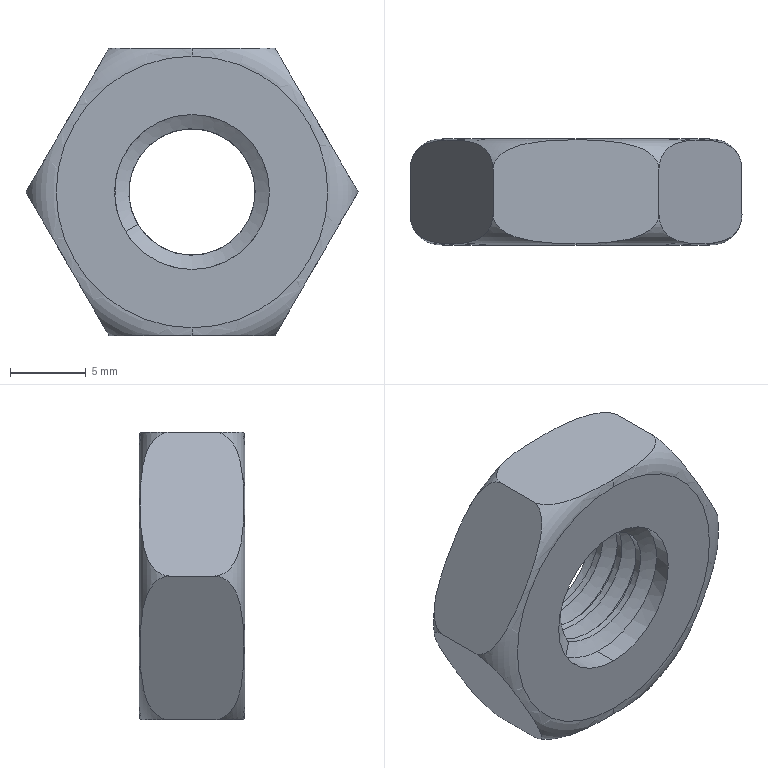Part | NX | features solid 2 | 1 solid | 25 faces | box 21.939 x 7 x 19 mm | volume 1677 mm3 | plane 10 | cylinder 8 | torus 4 | spline 3 | commonest cylinder face diameters 10.25 x8